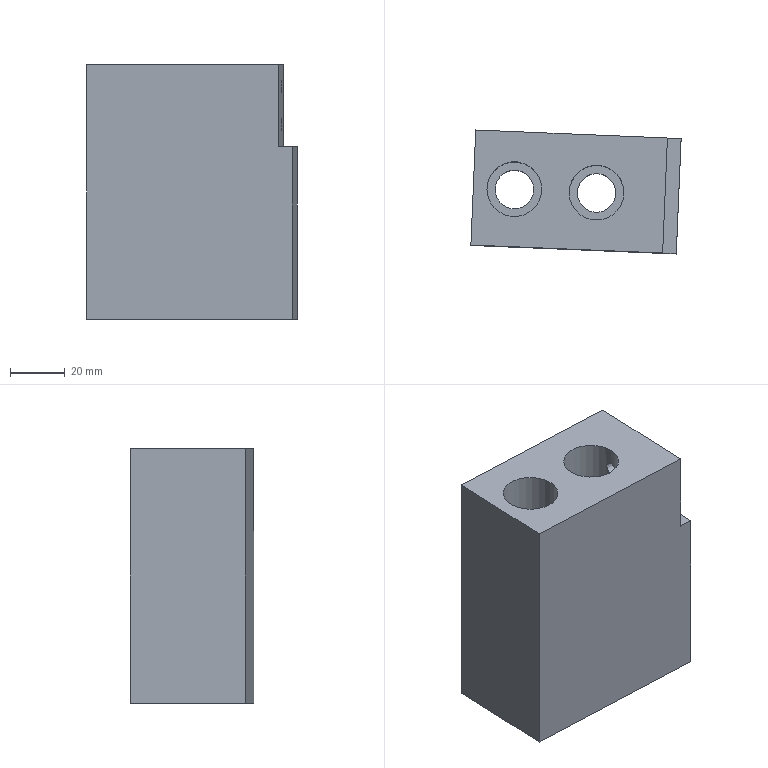Part | NX | features solid 2 | 1 solid | 16 faces | box 76.692 x 45.101 x 93 mm | volume 237260 mm3 | plane 10 | cylinder 6 | commonest cylinder face diameters 4.3 x2 14.1 x2 20 x2
STEP:
#1=CARTESIAN_POINT('',(3666.022,-344.374,-35.));
#2=VERTEX_POINT('',#1);
#3=CARTESIAN_POINT('',(3656.022,-344.374,-35.));
#4=DIRECTION('',(0.,0.,1.));
#5=DIRECTION('',(1.,0.,0.));
#6=AXIS2_PLACEMENT_3D('',#3,#4,#5);
#7=CIRCLE('',#6,10.);
#8=EDGE_CURVE('',#2,#2,#7,.T.);
#9=ORIENTED_EDGE('',*,*,#8,.F.);
#10=EDGE_LOOP('',(#9));
#11=FACE_BOUND('',#10,.T.);
#12=CARTESIAN_POINT('',(3680.121,-366.402,-35.));
#13=VERTEX_POINT('',#12);
#14=CARTESIAN_POINT('',(3681.879,-324.438,-35.));
#15=VERTEX_POINT('',#14);
#16=CARTESIAN_POINT('',(3681.,-345.42,-35.));
#17=DIRECTION('',(0.04184,0.9991,0.));
#18=VECTOR('',#17,1000.);
#19=LINE('',#16,#18);
#20=EDGE_CURVE('',#13,#15,#19,.T.);
#21=ORIENTED_EDGE('',*,*,#20,.T.);
#22=CARTESIAN_POINT('',(3611.94,-321.51,-35.));
#23=VERTEX_POINT('',#22);
#24=CARTESIAN_POINT('',(3641.914,-322.765,-35.));
#25=DIRECTION('',(0.9991,-0.04184,0.));
#26=VECTOR('',#25,1000.);
#27=LINE('',#24,#26);
#28=EDGE_CURVE('',#23,#15,#27,.T.);
#29=ORIENTED_EDGE('',*,*,#28,.F.);
#30=CARTESIAN_POINT('',(3610.183,-363.473,-35.));
#31=VERTEX_POINT('',#30);
#32=CARTESIAN_POINT('',(3611.061,-342.491,-35.));
#33=DIRECTION('',(0.04184,0.9991,0.));
#34=VECTOR('',#33,1000.);
#35=LINE('',#32,#34);
#36=EDGE_CURVE('',#31,#23,#35,.T.);
#37=ORIENTED_EDGE('',*,*,#36,.F.);
#38=CARTESIAN_POINT('',(3640.156,-364.728,-35.));
#39=DIRECTION('',(0.9991,-0.04184,0.));
#40=VECTOR('',#39,1000.);
#41=LINE('',#38,#40);
#42=EDGE_CURVE('',#31,#13,#41,.T.);
#43=ORIENTED_EDGE('',*,*,#42,.T.);
#44=EDGE_LOOP('',(#21,#29,#37,#43));
#45=FACE_BOUND('',#44,.T.);
#46=CARTESIAN_POINT('',(3636.048,-343.119,-35.));
#47=VERTEX_POINT('',#46);
#48=CARTESIAN_POINT('',(3626.048,-343.119,-35.));
#49=DIRECTION('',(0.,0.,1.));
#50=DIRECTION('',(1.,0.,0.));
#51=AXIS2_PLACEMENT_3D('',#48,#49,#50);
#52=CIRCLE('',#51,10.);
#53=EDGE_CURVE('',#47,#47,#52,.T.);
#54=ORIENTED_EDGE('',*,*,#53,.F.);
#55=EDGE_LOOP('',(#54));
#56=FACE_BOUND('',#55,.T.);
#57=CARTESIAN_POINT('',(3641.035,-343.746,-35.));
#58=DIRECTION('',(0.,0.,1.));
#59=DIRECTION('',(-1.,0.,0.));
#60=AXIS2_PLACEMENT_3D('',#57,#58,#59);
#61=PLANE('',#60);
#62=ADVANCED_FACE('',(#11,#45,#56),#61,.T.);
#63=CARTESIAN_POINT('',(3648.972,-344.374,-128.));
#64=VERTEX_POINT('',#63);
#65=CARTESIAN_POINT('',(3656.022,-344.374,-128.));
#66=DIRECTION('',(0.,0.,-1.));
#67=DIRECTION('',(-1.,0.,0.));
#68=AXIS2_PLACEMENT_3D('',#65,#66,#67);
#69=CIRCLE('',#68,7.05);
#70=EDGE_CURVE('',#64,#64,#69,.T.);
#71=ORIENTED_EDGE('',*,*,#70,.F.);
#72=EDGE_LOOP('',(#71));
#73=FACE_BOUND('',#72,.T.);
#74=CARTESIAN_POINT('',(3686.874,-324.647,-128.));
#75=VERTEX_POINT('',#74);
#76=CARTESIAN_POINT('',(3685.117,-366.611,-128.));
#77=VERTEX_POINT('',#76);
#78=CARTESIAN_POINT('',(3686.418,-335.539,-128.));
#79=DIRECTION('',(-0.04184,-0.9991,0.));
#80=VECTOR('',#79,1000.);
#81=LINE('',#78,#80);
#82=EDGE_CURVE('',#75,#77,#81,.T.);
#83=ORIENTED_EDGE('',*,*,#82,.T.);
#84=CARTESIAN_POINT('',(3610.183,-363.473,-128.));
#85=VERTEX_POINT('',#84);
#86=CARTESIAN_POINT('',(3640.156,-364.728,-128.));
#87=DIRECTION('',(0.9991,-0.04184,0.));
#88=VECTOR('',#87,1000.);
#89=LINE('',#86,#88);
#90=EDGE_CURVE('',#85,#77,#89,.T.);
#91=ORIENTED_EDGE('',*,*,#90,.F.);
#92=CARTESIAN_POINT('',(3611.94,-321.51,-128.));
#93=VERTEX_POINT('',#92);
#94=CARTESIAN_POINT('',(3611.484,-332.401,-128.));
#95=DIRECTION('',(-0.04184,-0.9991,0.));
#96=VECTOR('',#95,1000.);
#97=LINE('',#94,#96);
#98=EDGE_CURVE('',#93,#85,#97,.T.);
#99=ORIENTED_EDGE('',*,*,#98,.F.);
#100=CARTESIAN_POINT('',(3641.914,-322.765,-128.));
#101=DIRECTION('',(0.9991,-0.04184,0.));
#102=VECTOR('',#101,1000.);
#103=LINE('',#100,#102);
#104=EDGE_CURVE('',#93,#75,#103,.T.);
#105=ORIENTED_EDGE('',*,*,#104,.T.);
#106=EDGE_LOOP('',(#83,#91,#99,#105));
#107=FACE_BOUND('',#106,.T.);
#108=CARTESIAN_POINT('',(3618.998,-343.119,-128.));
#109=VERTEX_POINT('',#108);
#110=CARTESIAN_POINT('',(3626.048,-343.119,-128.));
#111=DIRECTION('',(0.,0.,-1.));
#112=DIRECTION('',(-1.,0.,0.));
#113=AXIS2_PLACEMENT_3D('',#110,#111,#112);
#114=CIRCLE('',#113,7.05);
#115=EDGE_CURVE('',#109,#109,#114,.T.);
#116=ORIENTED_EDGE('',*,*,#115,.F.);
#117=EDGE_LOOP('',(#116));
#118=FACE_BOUND('',#117,.T.);
#119=CARTESIAN_POINT('',(282.5,-193.,-128.));
#120=DIRECTION('',(0.,0.,-1.));
#121=DIRECTION('',(-1.,0.,0.));
#122=AXIS2_PLACEMENT_3D('',#119,#120,#121);
#123=PLANE('',#122);
#124=ADVANCED_FACE('',(#73,#107,#118),#123,.T.);
#125=CARTESIAN_POINT('',(3611.94,-321.51,-50.));
#126=DIRECTION('',(0.,0.,-1.));
#127=VECTOR('',#126,1000.);
#128=LINE('',#125,#127);
#129=EDGE_CURVE('',#23,#93,#128,.T.);
#130=ORIENTED_EDGE('',*,*,#129,.F.);
#131=ORIENTED_EDGE('',*,*,#28,.T.);
#132=CARTESIAN_POINT('',(3681.879,-324.438,-65.));
#133=VERTEX_POINT('',#132);
#134=CARTESIAN_POINT('',(3681.879,-324.438,-50.));
#135=DIRECTION('',(0.,0.,-1.));
#136=VECTOR('',#135,1000.);
#137=LINE('',#134,#136);
#138=EDGE_CURVE('',#15,#133,#137,.T.);
#139=ORIENTED_EDGE('',*,*,#138,.T.);
#140=CARTESIAN_POINT('',(3686.874,-324.647,-65.));
#141=VERTEX_POINT('',#140);
#142=CARTESIAN_POINT('',(3686.375,-324.627,-65.));
#143=DIRECTION('',(-0.9991,0.04184,0.));
#144=VECTOR('',#143,1000.);
#145=LINE('',#142,#144);
#146=EDGE_CURVE('',#141,#133,#145,.T.);
#147=ORIENTED_EDGE('',*,*,#146,.F.);
#148=CARTESIAN_POINT('',(3686.874,-324.647,-50.));
#149=DIRECTION('',(0.,0.,-1.));
#150=VECTOR('',#149,1000.);
#151=LINE('',#148,#150);
#152=EDGE_CURVE('',#141,#75,#151,.T.);
#153=ORIENTED_EDGE('',*,*,#152,.T.);
#154=ORIENTED_EDGE('',*,*,#104,.F.);
#155=EDGE_LOOP('',(#130,#131,#139,#147,#153,#154));
#156=FACE_BOUND('',#155,.T.);
#157=CARTESIAN_POINT('',(3641.914,-322.765,-50.));
#158=DIRECTION('',(0.04184,0.9991,0.));
#159=DIRECTION('',(-0.9991,0.04184,0.));
#160=AXIS2_PLACEMENT_3D('',#157,#158,#159);
#161=PLANE('',#160);
#162=ADVANCED_FACE('',(#156),#161,.T.);
#163=CARTESIAN_POINT('',(3680.121,-366.402,-65.));
#164=VERTEX_POINT('',#163);
#165=CARTESIAN_POINT('',(3680.121,-366.402,-50.));
#166=DIRECTION('',(0.,0.,-1.));
#167=VECTOR('',#166,1000.);
#168=LINE('',#165,#167);
#169=EDGE_CURVE('',#13,#164,#168,.T.);
#170=ORIENTED_EDGE('',*,*,#169,.F.);
#171=ORIENTED_EDGE('',*,*,#42,.F.);
#172=CARTESIAN_POINT('',(3610.183,-363.473,-50.));
#173=DIRECTION('',(0.,0.,-1.));
#174=VECTOR('',#173,1000.);
#175=LINE('',#172,#174);
#176=EDGE_CURVE('',#31,#85,#175,.T.);
#177=ORIENTED_EDGE('',*,*,#176,.T.);
#178=ORIENTED_EDGE('',*,*,#90,.T.);
#179=CARTESIAN_POINT('',(3685.117,-366.611,-65.));
#180=VERTEX_POINT('',#179);
#181=CARTESIAN_POINT('',(3685.117,-366.611,-50.));
#182=DIRECTION('',(0.,0.,-1.));
#183=VECTOR('',#182,1000.);
#184=LINE('',#181,#183);
#185=EDGE_CURVE('',#180,#77,#184,.T.);
#186=ORIENTED_EDGE('',*,*,#185,.F.);
#187=CARTESIAN_POINT('',(3684.618,-366.59,-65.));
#188=DIRECTION('',(-0.9991,0.04184,0.));
#189=VECTOR('',#188,1000.);
#190=LINE('',#187,#189);
#191=EDGE_CURVE('',#180,#164,#190,.T.);
#192=ORIENTED_EDGE('',*,*,#191,.T.);
#193=EDGE_LOOP('',(#170,#171,#177,#178,#186,#192));
#194=FACE_BOUND('',#193,.T.);
#195=CARTESIAN_POINT('',(3640.156,-364.728,-50.));
#196=DIRECTION('',(0.04184,0.9991,0.));
#197=DIRECTION('',(-0.9991,0.04184,0.));
#198=AXIS2_PLACEMENT_3D('',#195,#196,#197);
#199=PLANE('',#198);
#200=ADVANCED_FACE('',(#194),#199,.F.);
#201=ORIENTED_EDGE('',*,*,#176,.F.);
#202=ORIENTED_EDGE('',*,*,#36,.T.);
#203=ORIENTED_EDGE('',*,*,#129,.T.);
#204=ORIENTED_EDGE('',*,*,#98,.T.);
#205=EDGE_LOOP('',(#201,#202,#203,#204));
#206=FACE_BOUND('',#205,.T.);
#207=CARTESIAN_POINT('',(3611.061,-342.491,-50.));
#208=DIRECTION('',(-0.9991,0.04184,0.));
#209=DIRECTION('',(0.04184,0.9991,0.));
#210=AXIS2_PLACEMENT_3D('',#207,#208,#209);
#211=PLANE('',#210);
#212=ADVANCED_FACE('',(#206),#211,.T.);
#213=CARTESIAN_POINT('',(3681.004,-345.33,-54.852));
#214=VERTEX_POINT('',#213);
#215=CARTESIAN_POINT('',(3681.,-345.42,-57.));
#216=DIRECTION('',(-0.9991,0.04184,0.));
#217=DIRECTION('',(0.00175,0.0418,0.9991));
#218=AXIS2_PLACEMENT_3D('',#215,#216,#217);
#219=CIRCLE('',#218,2.15);
#220=EDGE_CURVE('',#214,#214,#219,.T.);
#221=ORIENTED_EDGE('',*,*,#220,.T.);
#222=EDGE_LOOP('',(#221));
#223=FACE_BOUND('',#222,.T.);
#224=CARTESIAN_POINT('',(3681.004,-345.33,-40.852));
#225=VERTEX_POINT('',#224);
#226=CARTESIAN_POINT('',(3681.,-345.42,-43.));
#227=DIRECTION('',(-0.9991,0.04184,0.));
#228=DIRECTION('',(0.00175,0.0418,0.9991));
#229=AXIS2_PLACEMENT_3D('',#226,#227,#228);
#230=CIRCLE('',#229,2.15);
#231=EDGE_CURVE('',#225,#225,#230,.T.);
#232=ORIENTED_EDGE('',*,*,#231,.T.);
#233=EDGE_LOOP('',(#232));
#234=FACE_BOUND('',#233,.T.);
#235=CARTESIAN_POINT('',(3681.,-345.42,-65.));
#236=DIRECTION('',(-0.04184,-0.9991,0.));
#237=VECTOR('',#236,1000.);
#238=LINE('',#235,#237);
#239=EDGE_CURVE('',#133,#164,#238,.T.);
#240=ORIENTED_EDGE('',*,*,#239,.F.);
#241=ORIENTED_EDGE('',*,*,#138,.F.);
#242=ORIENTED_EDGE('',*,*,#20,.F.);
#243=ORIENTED_EDGE('',*,*,#169,.T.);
#244=EDGE_LOOP('',(#240,#241,#242,#243));
#245=FACE_BOUND('',#244,.T.);
#246=CARTESIAN_POINT('',(3681.,-345.42,-50.));
#247=DIRECTION('',(-0.9991,0.04184,0.));
#248=DIRECTION('',(0.04184,0.9991,0.));
#249=AXIS2_PLACEMENT_3D('',#246,#247,#248);
#250=PLANE('',#249);
#251=ADVANCED_FACE('',(#223,#234,#245),#250,.F.);
#252=ORIENTED_EDGE('',*,*,#185,.T.);
#253=ORIENTED_EDGE('',*,*,#82,.F.);
#254=ORIENTED_EDGE('',*,*,#152,.F.);
#255=CARTESIAN_POINT('',(3685.996,-345.629,-65.));
#256=DIRECTION('',(0.04184,0.9991,0.));
#257=VECTOR('',#256,1000.);
#258=LINE('',#255,#257);
#259=EDGE_CURVE('',#180,#141,#258,.T.);
#260=ORIENTED_EDGE('',*,*,#259,.F.);
#261=EDGE_LOOP('',(#252,#253,#254,#260));
#262=FACE_BOUND('',#261,.T.);
#263=CARTESIAN_POINT('',(3685.996,-345.629,-50.));
#264=DIRECTION('',(-0.9991,0.04184,0.));
#265=DIRECTION('',(0.04184,0.9991,0.));
#266=AXIS2_PLACEMENT_3D('',#263,#264,#265);
#267=PLANE('',#266);
#268=ADVANCED_FACE('',(#262),#267,.F.);
#269=ORIENTED_EDGE('',*,*,#239,.T.);
#270=ORIENTED_EDGE('',*,*,#191,.F.);
#271=ORIENTED_EDGE('',*,*,#259,.T.);
#272=ORIENTED_EDGE('',*,*,#146,.T.);
#273=EDGE_LOOP('',(#269,#270,#271,#272));
#274=FACE_BOUND('',#273,.T.);
#275=CARTESIAN_POINT('',(3685.496,-345.608,-65.));
#276=DIRECTION('',(0.,0.,-1.));
#277=DIRECTION('',(1.,0.,0.));
#278=AXIS2_PLACEMENT_3D('',#275,#276,#277);
#279=PLANE('',#278);
#280=ADVANCED_FACE('',(#274),#279,.F.);
#281=CARTESIAN_POINT('',(3648.972,-344.374,-98.));
#282=VERTEX_POINT('',#281);
#283=CARTESIAN_POINT('',(3656.022,-344.374,-98.));
#284=DIRECTION('',(0.,0.,1.));
#285=DIRECTION('',(-1.,0.,0.));
#286=AXIS2_PLACEMENT_3D('',#283,#284,#285);
#287=CIRCLE('',#286,7.05);
#288=EDGE_CURVE('',#282,#282,#287,.T.);
#289=ORIENTED_EDGE('',*,*,#288,.T.);
#290=EDGE_LOOP('',(#289));
#291=FACE_BOUND('',#290,.T.);
#292=ORIENTED_EDGE('',*,*,#70,.T.);
#293=EDGE_LOOP('',(#292));
#294=FACE_BOUND('',#293,.T.);
#295=CARTESIAN_POINT('',(3656.022,-344.374,-35.));
#296=DIRECTION('',(0.,0.,-1.));
#297=DIRECTION('',(-1.,0.,0.));
#298=AXIS2_PLACEMENT_3D('',#295,#296,#297);
#299=CYLINDRICAL_SURFACE('',#298,7.05);
#300=ADVANCED_FACE('',(#291,#294),#299,.F.);
#301=ORIENTED_EDGE('',*,*,#288,.F.);
#302=EDGE_LOOP('',(#301));
#303=FACE_BOUND('',#302,.T.);
#304=CARTESIAN_POINT('',(3646.022,-344.374,-98.));
#305=VERTEX_POINT('',#304);
#306=CARTESIAN_POINT('',(3656.022,-344.374,-98.));
#307=DIRECTION('',(0.,0.,1.));
#308=DIRECTION('',(-1.,0.,0.));
#309=AXIS2_PLACEMENT_3D('',#306,#307,#308);
#310=CIRCLE('',#309,10.);
#311=EDGE_CURVE('',#305,#305,#310,.T.);
#312=ORIENTED_EDGE('',*,*,#311,.T.);
#313=EDGE_LOOP('',(#312));
#314=FACE_BOUND('',#313,.T.);
#315=CARTESIAN_POINT('',(3656.022,-344.374,-98.));
#316=DIRECTION('',(0.,0.,-1.));
#317=DIRECTION('',(1.,0.,0.));
#318=AXIS2_PLACEMENT_3D('',#315,#316,#317);
#319=PLANE('',#318);
#320=ADVANCED_FACE('',(#303,#314),#319,.F.);
#321=CARTESIAN_POINT('',(3666.022,-344.374,-54.891));
#322=VERTEX_POINT('',#321);
#323=CARTESIAN_POINT('',(3665.913,-342.807,-55.674));
#324=CARTESIAN_POINT('',(3666.077,-344.33,-54.662));
#325=CARTESIAN_POINT('',(3665.908,-346.118,-55.023));
#326=CARTESIAN_POINT('',(3665.636,-347.115,-56.533));
#327=CARTESIAN_POINT('',(3665.748,-346.762,-58.328));
#328=CARTESIAN_POINT('',(3666.038,-345.259,-59.336));
#329=CARTESIAN_POINT('',(3666.02,-343.466,-58.98));
#330=CARTESIAN_POINT('',(3665.832,-342.446,-57.466));
#331=CARTESIAN_POINT('',(3665.913,-342.807,-55.674));
#332=CARTESIAN_POINT('',(3666.077,-344.33,-54.662));
#333=CARTESIAN_POINT('',(3665.908,-346.118,-55.023));
#334=B_SPLINE_CURVE_WITH_KNOTS('',3,(#323,#324,#325,#326,#327,#328,#329,#330,#331,#332,#333),.UNSPECIFIED.,.T.,.F.,(1,1,1,1,1,1,1,1,1,1,1,1,1,1,1),(-0.005056,-0.003371,-0.001685,0.,0.001685,0.003371,0.005056,0.006741,0.008427,0.01011,0.0118,0.01348,0.01517,0.01685,0.01854),.UNSPECIFIED.);
#335=EDGE_CURVE('',#322,#322,#334,.T.);
#336=ORIENTED_EDGE('',*,*,#335,.T.);
#337=EDGE_LOOP('',(#336));
#338=FACE_BOUND('',#337,.T.);
#339=CARTESIAN_POINT('',(3666.022,-344.374,-40.891));
#340=VERTEX_POINT('',#339);
#341=CARTESIAN_POINT('',(3665.913,-342.807,-41.674));
#342=CARTESIAN_POINT('',(3666.077,-344.33,-40.662));
#343=CARTESIAN_POINT('',(3665.908,-346.118,-41.023));
#344=CARTESIAN_POINT('',(3665.636,-347.115,-42.533));
#345=CARTESIAN_POINT('',(3665.748,-346.762,-44.328));
#346=CARTESIAN_POINT('',(3666.038,-345.259,-45.336));
#347=CARTESIAN_POINT('',(3666.02,-343.466,-44.98));
#348=CARTESIAN_POINT('',(3665.832,-342.446,-43.466));
#349=CARTESIAN_POINT('',(3665.913,-342.807,-41.674));
#350=CARTESIAN_POINT('',(3666.077,-344.33,-40.662));
#351=CARTESIAN_POINT('',(3665.908,-346.118,-41.023));
#352=B_SPLINE_CURVE_WITH_KNOTS('',3,(#341,#342,#343,#344,#345,#346,#347,#348,#349,#350,#351),.UNSPECIFIED.,.T.,.F.,(1,1,1,1,1,1,1,1,1,1,1,1,1,1,1),(-0.005056,-0.003371,-0.001685,0.,0.001685,0.003371,0.005056,0.006741,0.008427,0.01011,0.0118,0.01348,0.01517,0.01685,0.01854),.UNSPECIFIED.);
#353=EDGE_CURVE('',#340,#340,#352,.T.);
#354=ORIENTED_EDGE('',*,*,#353,.T.);
#355=EDGE_LOOP('',(#354));
#356=FACE_BOUND('',#355,.T.);
#357=ORIENTED_EDGE('',*,*,#311,.F.);
#358=EDGE_LOOP('',(#357));
#359=FACE_BOUND('',#358,.T.);
#360=ORIENTED_EDGE('',*,*,#8,.T.);
#361=EDGE_LOOP('',(#360));
#362=FACE_BOUND('',#361,.T.);
#363=CARTESIAN_POINT('',(3656.022,-344.374,-35.));
#364=DIRECTION('',(0.,0.,-1.));
#365=DIRECTION('',(-1.,0.,0.));
#366=AXIS2_PLACEMENT_3D('',#363,#364,#365);
#367=CYLINDRICAL_SURFACE('',#366,10.);
#368=ADVANCED_FACE('',(#338,#356,#359,#362),#367,.F.);
#369=CARTESIAN_POINT('',(3618.998,-343.119,-98.));
#370=VERTEX_POINT('',#369);
#371=CARTESIAN_POINT('',(3626.048,-343.119,-98.));
#372=DIRECTION('',(0.,0.,1.));
#373=DIRECTION('',(-1.,0.,0.));
#374=AXIS2_PLACEMENT_3D('',#371,#372,#373);
#375=CIRCLE('',#374,7.05);
#376=EDGE_CURVE('',#370,#370,#375,.T.);
#377=ORIENTED_EDGE('',*,*,#376,.T.);
#378=EDGE_LOOP('',(#377));
#379=FACE_BOUND('',#378,.T.);
#380=ORIENTED_EDGE('',*,*,#115,.T.);
#381=EDGE_LOOP('',(#380));
#382=FACE_BOUND('',#381,.T.);
#383=CARTESIAN_POINT('',(3626.048,-343.119,-35.));
#384=DIRECTION('',(0.,0.,-1.));
#385=DIRECTION('',(-1.,0.,0.));
#386=AXIS2_PLACEMENT_3D('',#383,#384,#385);
#387=CYLINDRICAL_SURFACE('',#386,7.05);
#388=ADVANCED_FACE('',(#379,#382),#387,.F.);
#389=ORIENTED_EDGE('',*,*,#376,.F.);
#390=EDGE_LOOP('',(#389));
#391=FACE_BOUND('',#390,.T.);
#392=CARTESIAN_POINT('',(3616.048,-343.119,-98.));
#393=VERTEX_POINT('',#392);
#394=CARTESIAN_POINT('',(3626.048,-343.119,-98.));
#395=DIRECTION('',(0.,0.,1.));
#396=DIRECTION('',(-1.,0.,0.));
#397=AXIS2_PLACEMENT_3D('',#394,#395,#396);
#398=CIRCLE('',#397,10.);
#399=EDGE_CURVE('',#393,#393,#398,.T.);
#400=ORIENTED_EDGE('',*,*,#399,.T.);
#401=EDGE_LOOP('',(#400));
#402=FACE_BOUND('',#401,.T.);
#403=CARTESIAN_POINT('',(3656.022,-344.374,-98.));
#404=DIRECTION('',(0.,0.,-1.));
#405=DIRECTION('',(1.,0.,0.));
#406=AXIS2_PLACEMENT_3D('',#403,#404,#405);
#407=PLANE('',#406);
#408=ADVANCED_FACE('',(#391,#402),#407,.F.);
#409=ORIENTED_EDGE('',*,*,#399,.F.);
#410=EDGE_LOOP('',(#409));
#411=FACE_BOUND('',#410,.T.);
#412=ORIENTED_EDGE('',*,*,#53,.T.);
#413=EDGE_LOOP('',(#412));
#414=FACE_BOUND('',#413,.T.);
#415=CARTESIAN_POINT('',(3626.048,-343.119,-35.));
#416=DIRECTION('',(0.,0.,-1.));
#417=DIRECTION('',(-1.,0.,0.));
#418=AXIS2_PLACEMENT_3D('',#415,#416,#417);
#419=CYLINDRICAL_SURFACE('',#418,10.);
#420=ADVANCED_FACE('',(#411,#414),#419,.F.);
#421=ORIENTED_EDGE('',*,*,#231,.F.);
#422=EDGE_LOOP('',(#421));
#423=FACE_BOUND('',#422,.T.);
#424=ORIENTED_EDGE('',*,*,#353,.F.);
#425=EDGE_LOOP('',(#424));
#426=FACE_BOUND('',#425,.T.);
#427=CARTESIAN_POINT('',(3681.,-345.42,-43.));
#428=DIRECTION('',(-0.9991,0.04184,0.));
#429=DIRECTION('',(-0.00175,-0.0418,-0.9991));
#430=AXIS2_PLACEMENT_3D('',#427,#428,#429);
#431=CYLINDRICAL_SURFACE('',#430,2.15);
#432=ADVANCED_FACE('',(#423,#426),#431,.F.);
#433=ORIENTED_EDGE('',*,*,#220,.F.);
#434=EDGE_LOOP('',(#433));
#435=FACE_BOUND('',#434,.T.);
#436=ORIENTED_EDGE('',*,*,#335,.F.);
#437=EDGE_LOOP('',(#436));
#438=FACE_BOUND('',#437,.T.);
#439=CARTESIAN_POINT('',(3681.,-345.42,-57.));
#440=DIRECTION('',(-0.9991,0.04184,0.));
#441=DIRECTION('',(-0.00175,-0.0418,-0.9991));
#442=AXIS2_PLACEMENT_3D('',#439,#440,#441);
#443=CYLINDRICAL_SURFACE('',#442,2.15);
#444=ADVANCED_FACE('',(#435,#438),#443,.F.);
#445=CLOSED_SHELL('',(#62,#124,#162,#200,#212,#251,#268,#280,#300,#320,#368,#388,#408,#420,#432,#444));
#446=MANIFOLD_SOLID_BREP('',#445);
#447=(LENGTH_UNIT()NAMED_UNIT(*)SI_UNIT(.MILLI.,.METRE.));
#448=UNCERTAINTY_MEASURE_WITH_UNIT(LENGTH_MEASURE(0.0508),#447,'','');
#449=(NAMED_UNIT(*)PLANE_ANGLE_UNIT()SI_UNIT($,.RADIAN.));
#450=(NAMED_UNIT(*)SI_UNIT($,.STERADIAN.)SOLID_ANGLE_UNIT());
#451=(GEOMETRIC_REPRESENTATION_CONTEXT(3)GLOBAL_UNCERTAINTY_ASSIGNED_CONTEXT((#448))GLOBAL_UNIT_ASSIGNED_CONTEXT((#447,#449,#450))REPRESENTATION_CONTEXT('',''));
#452=ADVANCED_BREP_SHAPE_REPRESENTATION('',(#446),#451);